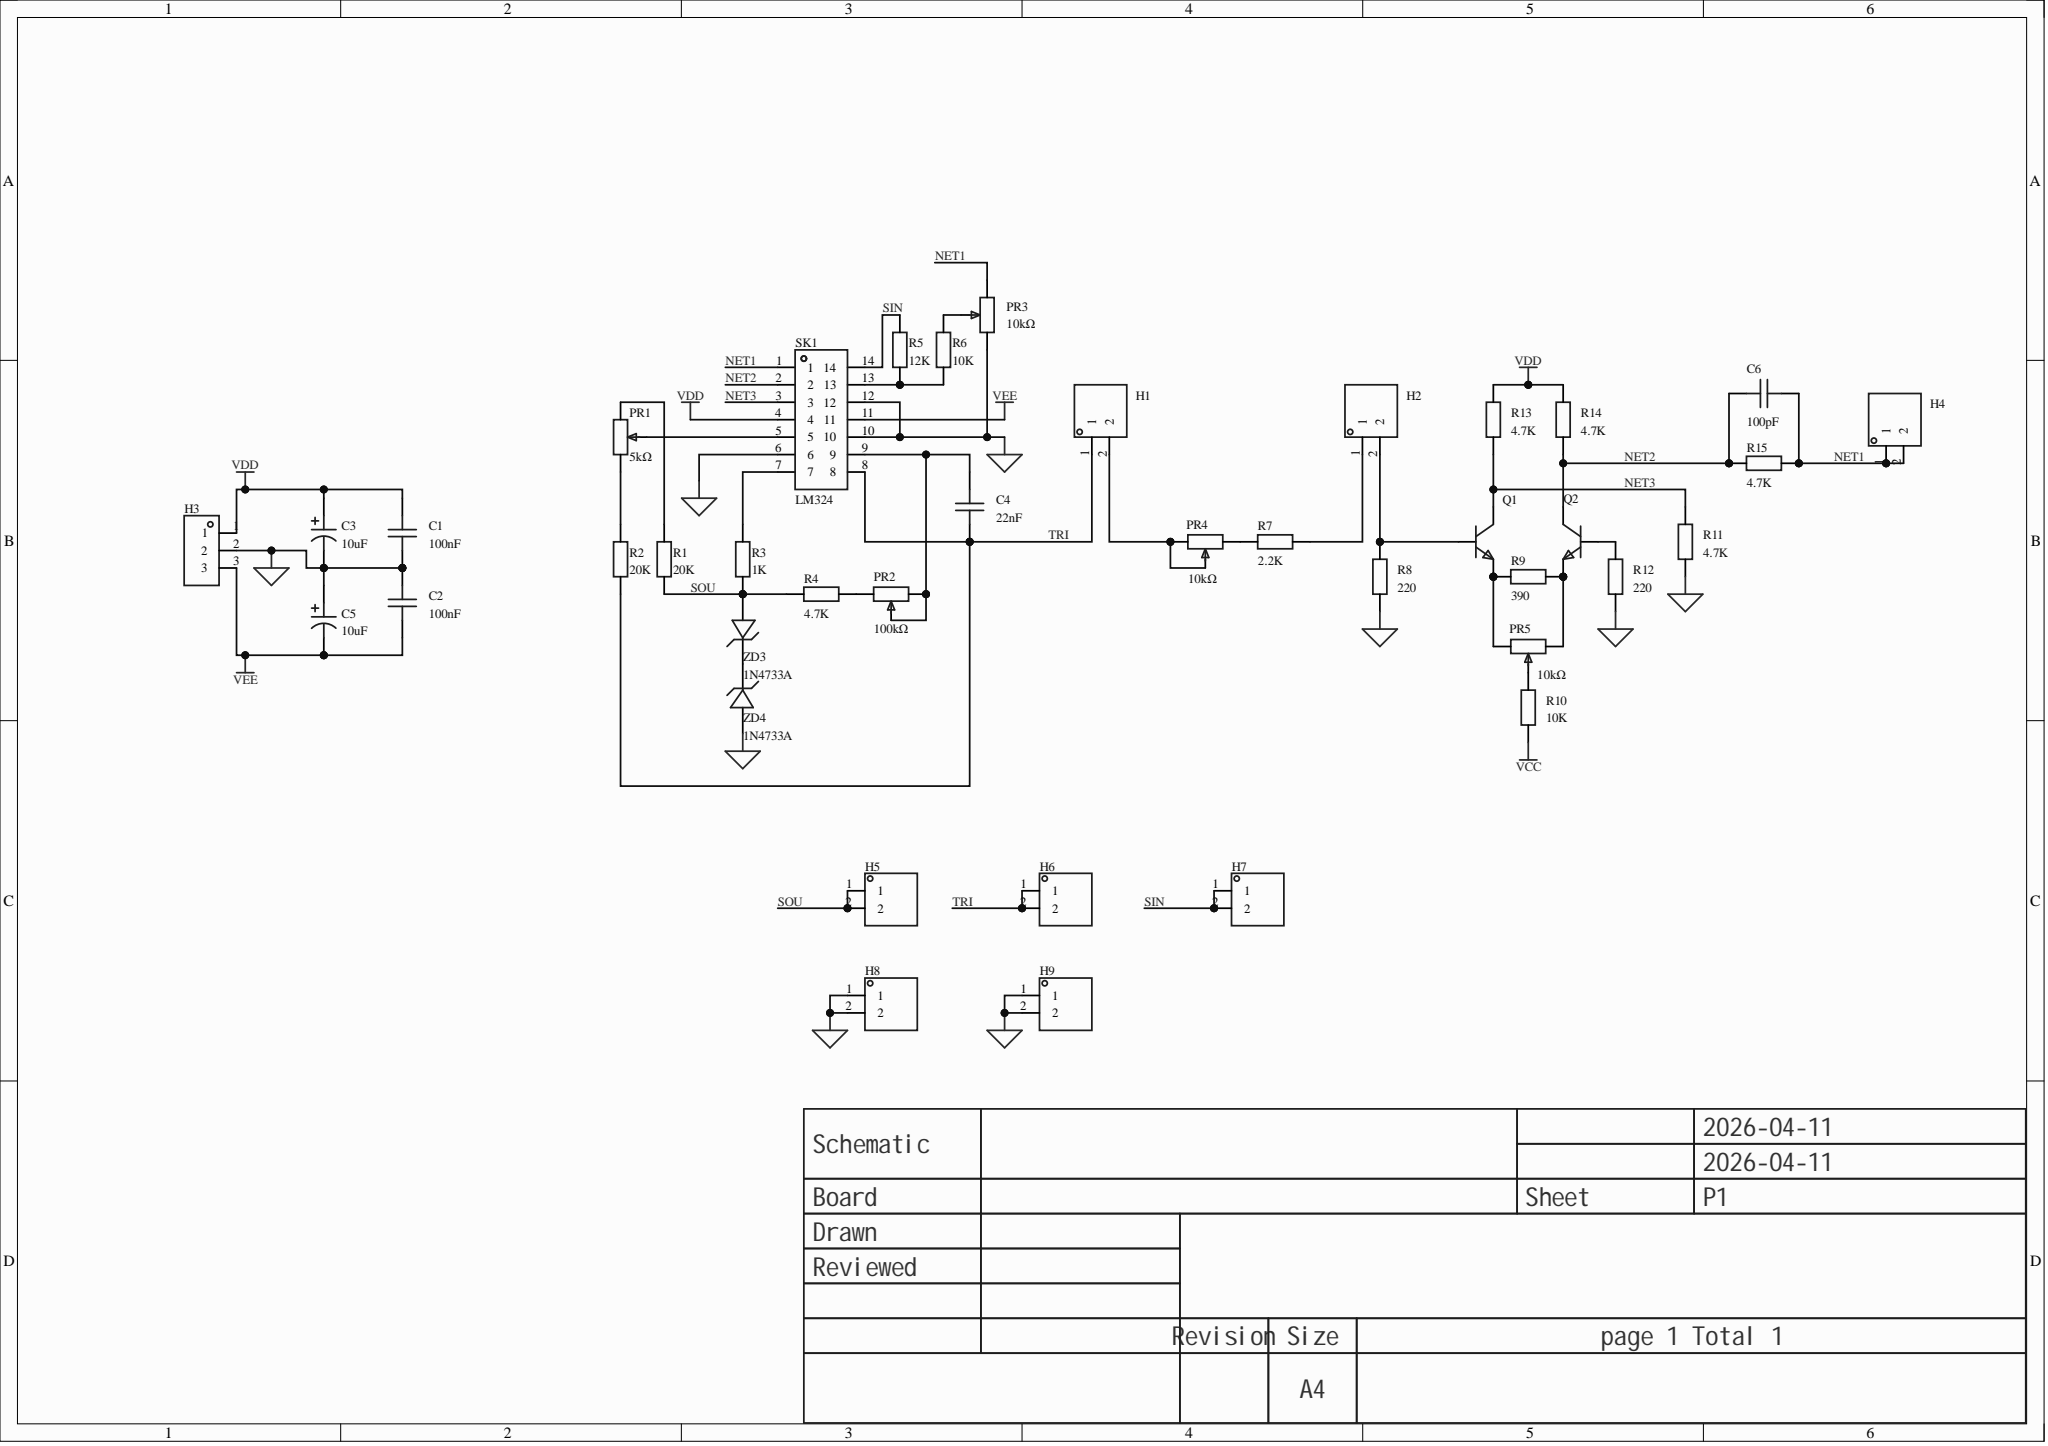Circuit board | Altium Designer | 40 parts | 26 nets
Bill of materials:
Comment,Description,Designator,Footprint,LibRef,Quantity
"100nF","","C1, C2","L0805","CAP_0603","2"
"10uF","Capacitance:10uF;Tolerance:±20%;Rated voltage:50V;Ripple current:180mA@100kHz;Equivalent series resistance (ESR):1.3Ω@100kHz;","C3, C5","CAP-TH_BD5.0-P2.00-D0.5-FD-A","ERG50V10M5X11","2"
"22nF","","C4","C0805","CAP_0805","1"
"100pF","","C6","C0805","CAP_0805","1"
"","","H1, H2, H4, H5, H6, H7, H8, H9","HDR-TH_2P-P2.54-V-M-1","HDR-M_2.54_1x2P","8"
"","","H3","CONN-TH_3P-P2.50_HX-XH2.54-3PZZ-B","HDR-M_2.54_1x3P","1"
"5kΩ","","PR1","R_3296","R_3296","1"
"100kΩ","","PR2","R_3296","R_3296","1"
"10kΩ","","PR3, PR4, PR5","R_3296","R_3296","3"
"","","Q1, Q2","S8050_TO_92","S8050_TO_NPN","2"
"20K","","R1, R2","R0805","Res_0805","2"
"1K","","R3","R0805","Res_0805","1"
"4.7K","","R4, R11, R13, R14, R15","R0805","Res_0805","5"
"12K","","R5","R0805","Res_0805","1"
"10K","","R6, R10","R0805","Res_0805","2"
"2.2K","","R7","R0805","Res_0805","1"
"220","","R8, R12","R0805","Res_0805","2"
"390","","R9","R0805","Res_0805","1"
"LM324","Adapted package type:DIP;Pitch:2.54mm;Row spacing:7.62mm;Round/square hole:Square hole;Total PIN count:14P;Contact plating:Tin;Operating temperature:-55℃~+105℃;","SK1","DIP-14_L17.8-W10.2-P2.54-BL","Z-ICS0S14P-NG00","1"
"1N4733A","Diode configuration:Single;Zener voltage (nominal):5.1V;Zener voltage (range):4.84V~5.36V;Power dissipation (Pd):1W;","ZD3, ZD4","DO-41_BD2.8-L4.2-P8.00-D0.7-FD","1N4733A","2"
Netlist (Protel format):
[
C1
L0805
100nF



]
[
C2
L0805
100nF



]
[
C3
CAP-TH_BD5.0-P2.00-D0.5-FD-A
10uF



]
[
C4
C0805
22nF



]
[
C5
CAP-TH_BD5.0-P2.00-D0.5-FD-A
10uF



]
[
C6
C0805
100pF



]
[
H1
HDR-TH_2P-P2.54-V-M-1




]
[
H2
HDR-TH_2P-P2.54-V-M-1




]
[
H3
CONN-TH_3P-P2.50_HX-XH2.54-3PZZ-B




]
[
H4
HDR-TH_2P-P2.54-V-M-1




]
[
H5
HDR-TH_2P-P2.54-V-M-1




]
[
H6
HDR-TH_2P-P2.54-V-M-1




]
[
H7
HDR-TH_2P-P2.54-V-M-1




]
[
H8
HDR-TH_2P-P2.54-V-M-1




]
[
H9
HDR-TH_2P-P2.54-V-M-1




]
[
PR1
R_3296
5kΩ



]
[
PR2
R_3296
100kΩ



]
[
PR3
R_3296
10kΩ



]
[
PR4
R_3296
10kΩ



]
[
PR5
R_3296
10kΩ



]
[
Q1
S8050_TO_92




]
[
Q2
S8050_TO_92




]
[
R1
R0805
20K



]
[
R2
R0805
20K



]
[
R3
R0805
1K



]
[
R4
R0805
4.7K



]
[
R5
R0805
12K



]
[
R6
R0805
10K



]
[
R7
R0805
2.2K



]
[
R8
R0805
220



]
[
R9
R0805
390



]
[
R10
R0805
10K



]
[
R11
R0805
4.7K



]
[
R12
R0805
220



]
[
R13
R0805
4.7K



]
[
R14
R0805
4.7K



]
[
R15
R0805
4.7K



]
[
SK1
DIP-14_L17.8-W10.2-P2.54-BL
LM324



]
[
ZD3
DO-41_BD2.8-L4.2-P8.00-D0.7-FD
1N4733A



]
[
ZD4
DO-41_BD2.8-L4.2-P8.00-D0.7-FD
1N4733A



]
(
VEE
C2-1
C5-2
H3-3
SK1-11
)
(
VDD
C1-2
C3-1
H3-1
R13-2
R14-2
SK1-4
)
(
TRI
C4-1
H1-1
H6-1
H6-2
R2-1
SK1-8
)
(
SOU
H5-1
H5-2
R1-1
R3-1
R4-2
ZD3-1
)
(
SIN
H7-1
H7-2
R5-2
SK1-14
)
(
NetZD3_2
ZD3-2
ZD4-2
)
(
NetR5_1
R5-1
R6-1
SK1-13
)
(
NetR3_2
R3-2
SK1-7
)
(
NetQ2_2
Q2-2
R12-2
)
(
NetPR5_3
PR5-3
Q2-1
R9-2
)
(
NetPR5_2
PR5-2
R10-2
)
(
NetPR5_1
PR5-1
Q1-1
R9-1
)
(
NetPR4_3
PR4-3
R7-1
)
(
NetPR3_2
PR3-2
R6-2
)
(
NetPR2_1
PR2-1
R4-1
)
(
NetPR1_3
PR1-3
R1-2
)
(
NetPR1_2
PR1-2
SK1-5
)
(
NetPR1_1
PR1-1
R2-2
)
(
NetH2_2
H2-2
Q1-2
R8-2
)
(
NetH2_1
H2-1
R7-2
)
(
NetH1_2
H1-2
PR4-1
PR4-2
)
(
NetC4_2
C4-2
PR2-2
PR2-3
SK1-9
)
(
NET3
Q1-3
R11-2
R13-1
SK1-3
)
(
NET2
C6-1
Q2-3
R14-1
R15-2
SK1-2
)
(
NET1
C6-2
H4-1
H4-2
PR3-1
R15-1
SK1-1
)
(
GND
C1-1
C2-2
C3-2
C5-1
H3-2
H8-1
H8-2
H9-1
H9-2
PR3-3
R8-1
R11-1
R12-1
SK1-6
SK1-10
SK1-12
ZD4-1
)